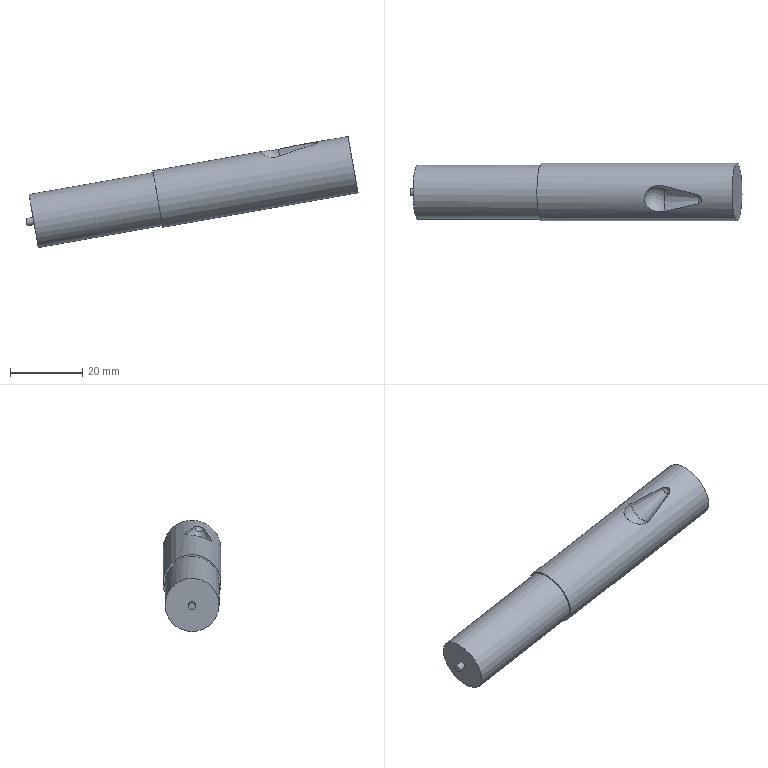Part | NX | features solid 2 | 1 solid | 10 faces | box 92.165 x 16 x 30.893 mm | volume 17061 mm3 | plane 4 | cylinder 3 | sphere 2 | cone 1 | commonest cylinder face diameters 2 x1 15 x1 16 x1
STEP:
#1=CARTESIAN_POINT('',(483.267,49.483,15.725));
#2=VERTEX_POINT('',#1);
#3=CARTESIAN_POINT('',(481.965,49.483,23.111));
#4=DIRECTION('',(-0.9848,0.,-0.1736));
#5=DIRECTION('',(0.1736,0.,-0.9848));
#6=AXIS2_PLACEMENT_3D('',#3,#4,#5);
#7=CIRCLE('',#6,7.5);
#8=EDGE_CURVE('',#2,#2,#7,.T.);
#9=ORIENTED_EDGE('',*,*,#8,.T.);
#10=EDGE_LOOP('',(#9));
#11=FACE_BOUND('',#10,.T.);
#12=CARTESIAN_POINT('',(482.139,49.483,22.126));
#13=VERTEX_POINT('',#12);
#14=CARTESIAN_POINT('',(481.965,49.483,23.111));
#15=DIRECTION('',(-0.9848,0.,-0.1736));
#16=DIRECTION('',(0.1736,0.,-0.9848));
#17=AXIS2_PLACEMENT_3D('',#14,#15,#16);
#18=CIRCLE('',#17,1.);
#19=EDGE_CURVE('',#13,#13,#18,.F.);
#20=ORIENTED_EDGE('',*,*,#19,.T.);
#21=EDGE_LOOP('',(#20));
#22=FACE_BOUND('',#21,.T.);
#23=CARTESIAN_POINT('',(481.965,49.483,23.111));
#24=DIRECTION('',(0.9848,0.,0.1736));
#25=DIRECTION('',(0.04494,-0.9659,-0.2549));
#26=AXIS2_PLACEMENT_3D('',#23,#24,#25);
#27=PLANE('',#26);
#28=ADVANCED_FACE('',(#11,#22),#27,.F.);
#29=CARTESIAN_POINT('',(550.214,44.025,41.085));
#30=VERTEX_POINT('',#29);
#31=CARTESIAN_POINT('',(559.811,46.196,44.244));
#32=VERTEX_POINT('',#31);
#33=CARTESIAN_POINT('',(550.214,44.025,41.085));
#34=CARTESIAN_POINT('',(553.389,44.673,42.258));
#35=CARTESIAN_POINT('',(556.587,45.408,43.315));
#36=CARTESIAN_POINT('',(559.811,46.196,44.244));
#37=B_SPLINE_CURVE_WITH_KNOTS('',3,(#33,#34,#35,#36),.UNSPECIFIED.,.F.,.F.,(4,4),(0.000000207,0.01034),.UNSPECIFIED.);
#38=EDGE_CURVE('',#30,#32,#37,.T.);
#39=ORIENTED_EDGE('',*,*,#38,.F.);
#40=CARTESIAN_POINT('',(549.876,51.284,43.));
#41=VERTEX_POINT('',#40);
#42=CARTESIAN_POINT('',(549.876,51.284,43.));
#43=CARTESIAN_POINT('',(548.717,51.593,42.723));
#44=CARTESIAN_POINT('',(546.764,51.174,42.546));
#45=CARTESIAN_POINT('',(545.188,49.214,42.441));
#46=CARTESIAN_POINT('',(544.811,47.399,42.113));
#47=CARTESIAN_POINT('',(545.35,45.687,41.51));
#48=CARTESIAN_POINT('',(547.089,44.077,40.674));
#49=CARTESIAN_POINT('',(549.08,43.793,40.665));
#50=CARTESIAN_POINT('',(550.214,44.025,41.085));
#51=B_SPLINE_CURVE_WITH_KNOTS('',3,(#42,#43,#44,#45,#46,#47,#48,#49,#50),.UNSPECIFIED.,.F.,.F.,(4,1,1,1,1,1,4),(0.000000204,0.003641,0.005462,0.007282,0.009103,0.01092,0.01456),.UNSPECIFIED.);
#52=EDGE_CURVE('',#41,#30,#51,.T.);
#53=ORIENTED_EDGE('',*,*,#52,.F.);
#54=CARTESIAN_POINT('',(559.696,48.682,44.9));
#55=VERTEX_POINT('',#54);
#56=CARTESIAN_POINT('',(559.696,48.682,44.9));
#57=CARTESIAN_POINT('',(556.395,49.542,44.405));
#58=CARTESIAN_POINT('',(553.122,50.421,43.775));
#59=CARTESIAN_POINT('',(549.876,51.284,43.));
#60=B_SPLINE_CURVE_WITH_KNOTS('',3,(#56,#57,#58,#59),.UNSPECIFIED.,.F.,.F.,(4,4),(0.000000207,0.01034),.UNSPECIFIED.);
#61=EDGE_CURVE('',#55,#41,#60,.T.);
#62=ORIENTED_EDGE('',*,*,#61,.F.);
#63=CARTESIAN_POINT('',(559.811,46.196,44.244));
#64=CARTESIAN_POINT('',(560.365,46.331,44.403));
#65=CARTESIAN_POINT('',(561.128,47.389,44.994));
#66=CARTESIAN_POINT('',(560.262,48.534,44.984));
#67=CARTESIAN_POINT('',(559.696,48.682,44.9));
#68=B_SPLINE_CURVE_WITH_KNOTS('',3,(#63,#64,#65,#66,#67),.UNSPECIFIED.,.F.,.F.,(4,1,4),(0.000000204,0.00175,0.003499),.UNSPECIFIED.);
#69=EDGE_CURVE('',#32,#55,#68,.T.);
#70=ORIENTED_EDGE('',*,*,#69,.F.);
#71=EDGE_LOOP('',(#39,#53,#62,#70));
#72=FACE_BOUND('',#71,.T.);
#73=CARTESIAN_POINT('',(570.957,41.755,36.7));
#74=VERTEX_POINT('',#73);
#75=CARTESIAN_POINT('',(570.598,49.483,38.739));
#76=DIRECTION('',(-0.9848,0.,-0.1736));
#77=DIRECTION('',(0.04494,-0.9659,-0.2549));
#78=AXIS2_PLACEMENT_3D('',#75,#76,#77);
#79=CIRCLE('',#78,8.);
#80=EDGE_CURVE('',#74,#74,#79,.T.);
#81=ORIENTED_EDGE('',*,*,#80,.T.);
#82=EDGE_LOOP('',(#81));
#83=FACE_BOUND('',#82,.T.);
#84=CARTESIAN_POINT('',(516.793,41.755,27.15));
#85=VERTEX_POINT('',#84);
#86=CARTESIAN_POINT('',(516.433,49.483,29.189));
#87=DIRECTION('',(-0.9848,0.,-0.1736));
#88=DIRECTION('',(0.04494,-0.9659,-0.2549));
#89=AXIS2_PLACEMENT_3D('',#86,#87,#88);
#90=CIRCLE('',#89,8.);
#91=EDGE_CURVE('',#85,#85,#90,.T.);
#92=ORIENTED_EDGE('',*,*,#91,.F.);
#93=EDGE_LOOP('',(#92));
#94=FACE_BOUND('',#93,.T.);
#95=CARTESIAN_POINT('',(570.598,49.483,38.739));
#96=DIRECTION('',(-0.9848,0.,-0.1736));
#97=DIRECTION('',(-0.04494,0.9659,0.2549));
#98=AXIS2_PLACEMENT_3D('',#95,#96,#97);
#99=CYLINDRICAL_SURFACE('',#98,8.);
#100=ADVANCED_FACE('',(#72,#83,#94),#99,.T.);
#101=ORIENTED_EDGE('',*,*,#80,.F.);
#102=EDGE_LOOP('',(#101));
#103=FACE_BOUND('',#102,.T.);
#104=CARTESIAN_POINT('',(570.598,49.483,38.739));
#105=DIRECTION('',(0.9848,0.,0.1736));
#106=DIRECTION('',(0.04494,-0.9659,-0.2549));
#107=AXIS2_PLACEMENT_3D('',#104,#105,#106);
#108=PLANE('',#107);
#109=ADVANCED_FACE('',(#103),#108,.T.);
#110=CARTESIAN_POINT('',(516.77,42.238,27.277));
#111=VERTEX_POINT('',#110);
#112=CARTESIAN_POINT('',(516.433,49.483,29.189));
#113=DIRECTION('',(-0.9848,0.,-0.1736));
#114=DIRECTION('',(0.04494,-0.9659,-0.2549));
#115=AXIS2_PLACEMENT_3D('',#112,#113,#114);
#116=CIRCLE('',#115,7.5);
#117=EDGE_CURVE('',#111,#111,#116,.T.);
#118=ORIENTED_EDGE('',*,*,#117,.F.);
#119=EDGE_LOOP('',(#118));
#120=FACE_BOUND('',#119,.T.);
#121=ORIENTED_EDGE('',*,*,#91,.T.);
#122=EDGE_LOOP('',(#121));
#123=FACE_BOUND('',#122,.T.);
#124=CARTESIAN_POINT('',(516.433,49.483,29.189));
#125=DIRECTION('',(0.9848,0.,0.1736));
#126=DIRECTION('',(0.04494,-0.9659,-0.2549));
#127=AXIS2_PLACEMENT_3D('',#124,#125,#126);
#128=PLANE('',#127);
#129=ADVANCED_FACE('',(#120,#123),#128,.F.);
#130=ORIENTED_EDGE('',*,*,#8,.F.);
#131=EDGE_LOOP('',(#130));
#132=FACE_BOUND('',#131,.T.);
#133=ORIENTED_EDGE('',*,*,#117,.T.);
#134=EDGE_LOOP('',(#133));
#135=FACE_BOUND('',#134,.T.);
#136=CARTESIAN_POINT('',(491.813,49.483,24.847));
#137=DIRECTION('',(0.9848,0.,0.1736));
#138=DIRECTION('',(0.04494,-0.9659,-0.2549));
#139=AXIS2_PLACEMENT_3D('',#136,#137,#138);
#140=CYLINDRICAL_SURFACE('',#139,7.5);
#141=ADVANCED_FACE('',(#132,#135),#140,.T.);
#142=CARTESIAN_POINT('',(549.888,47.412,42.934));
#143=DIRECTION('',(0.9848,0.,0.1736));
#144=DIRECTION('',(-0.04494,0.9659,0.2549));
#145=AXIS2_PLACEMENT_3D('',#142,#143,#144);
#146=CIRCLE('',#145,3.873);
#147=EDGE_CURVE('',#30,#41,#146,.T.);
#148=ORIENTED_EDGE('',*,*,#147,.T.);
#149=ORIENTED_EDGE('',*,*,#52,.T.);
#150=EDGE_LOOP('',(#148,#149));
#151=FACE_BOUND('',#150,.T.);
#152=CARTESIAN_POINT('',(548.903,47.412,42.761));
#153=DIRECTION('',(-0.9848,0.,-0.1736));
#154=DIRECTION('',(-0.04494,0.9659,0.2549));
#155=AXIS2_PLACEMENT_3D('',#152,#153,#154);
#156=SPHERICAL_SURFACE('',#155,4.);
#157=ADVANCED_FACE('',(#151),#156,.F.);
#158=CARTESIAN_POINT('',(559.736,47.412,44.671));
#159=DIRECTION('',(0.9848,0.,0.1736));
#160=DIRECTION('',(-0.04494,0.9659,0.2549));
#161=AXIS2_PLACEMENT_3D('',#158,#159,#160);
#162=CIRCLE('',#161,1.291);
#163=EDGE_CURVE('',#32,#55,#162,.T.);
#164=ORIENTED_EDGE('',*,*,#163,.T.);
#165=ORIENTED_EDGE('',*,*,#61,.T.);
#166=ORIENTED_EDGE('',*,*,#147,.F.);
#167=ORIENTED_EDGE('',*,*,#38,.T.);
#168=EDGE_LOOP('',(#164,#165,#166,#167));
#169=FACE_BOUND('',#168,.T.);
#170=CARTESIAN_POINT('',(549.888,47.412,42.934));
#171=DIRECTION('',(-0.9848,0.,-0.1736));
#172=DIRECTION('',(-0.04494,0.9659,0.2549));
#173=AXIS2_PLACEMENT_3D('',#170,#171,#172);
#174=CONICAL_SURFACE('',#173,3.873,0.2527);
#175=ADVANCED_FACE('',(#169),#174,.F.);
#176=ORIENTED_EDGE('',*,*,#163,.F.);
#177=ORIENTED_EDGE('',*,*,#69,.T.);
#178=EDGE_LOOP('',(#176,#177));
#179=FACE_BOUND('',#178,.T.);
#180=CARTESIAN_POINT('',(559.408,47.412,44.613));
#181=DIRECTION('',(-0.9848,0.,-0.1736));
#182=DIRECTION('',(0.04494,-0.9659,-0.2549));
#183=AXIS2_PLACEMENT_3D('',#180,#181,#182);
#184=SPHERICAL_SURFACE('',#183,1.333);
#185=ADVANCED_FACE('',(#179),#184,.F.);
#186=ORIENTED_EDGE('',*,*,#19,.F.);
#187=EDGE_LOOP('',(#186));
#188=FACE_BOUND('',#187,.T.);
#189=CARTESIAN_POINT('',(480.169,49.483,21.779));
#190=VERTEX_POINT('',#189);
#191=CARTESIAN_POINT('',(479.995,49.483,22.764));
#192=DIRECTION('',(-0.9848,0.,-0.1736));
#193=DIRECTION('',(0.1736,0.,-0.9848));
#194=AXIS2_PLACEMENT_3D('',#191,#192,#193);
#195=CIRCLE('',#194,1.);
#196=EDGE_CURVE('',#190,#190,#195,.T.);
#197=ORIENTED_EDGE('',*,*,#196,.F.);
#198=EDGE_LOOP('',(#197));
#199=FACE_BOUND('',#198,.T.);
#200=CARTESIAN_POINT('',(481.965,49.483,23.111));
#201=DIRECTION('',(-0.9848,0.,-0.1736));
#202=DIRECTION('',(-0.1736,0.,0.9848));
#203=AXIS2_PLACEMENT_3D('',#200,#201,#202);
#204=CYLINDRICAL_SURFACE('',#203,1.);
#205=ADVANCED_FACE('',(#188,#199),#204,.T.);
#206=ORIENTED_EDGE('',*,*,#196,.T.);
#207=EDGE_LOOP('',(#206));
#208=FACE_BOUND('',#207,.T.);
#209=CARTESIAN_POINT('',(479.995,49.483,22.764));
#210=DIRECTION('',(0.9848,0.,0.1736));
#211=DIRECTION('',(0.04494,-0.9659,-0.2549));
#212=AXIS2_PLACEMENT_3D('',#209,#210,#211);
#213=PLANE('',#212);
#214=ADVANCED_FACE('',(#208),#213,.F.);
#215=CLOSED_SHELL('',(#28,#100,#109,#129,#141,#157,#175,#185,#205,#214));
#216=MANIFOLD_SOLID_BREP('',#215);
#217=(LENGTH_UNIT()NAMED_UNIT(*)SI_UNIT(.MILLI.,.METRE.));
#218=UNCERTAINTY_MEASURE_WITH_UNIT(LENGTH_MEASURE(0.0508),#217,'','');
#219=(NAMED_UNIT(*)PLANE_ANGLE_UNIT()SI_UNIT($,.RADIAN.));
#220=(NAMED_UNIT(*)SI_UNIT($,.STERADIAN.)SOLID_ANGLE_UNIT());
#221=(GEOMETRIC_REPRESENTATION_CONTEXT(3)GLOBAL_UNCERTAINTY_ASSIGNED_CONTEXT((#218))GLOBAL_UNIT_ASSIGNED_CONTEXT((#217,#219,#220))REPRESENTATION_CONTEXT('',''));
#222=ADVANCED_BREP_SHAPE_REPRESENTATION('',(#216),#221);